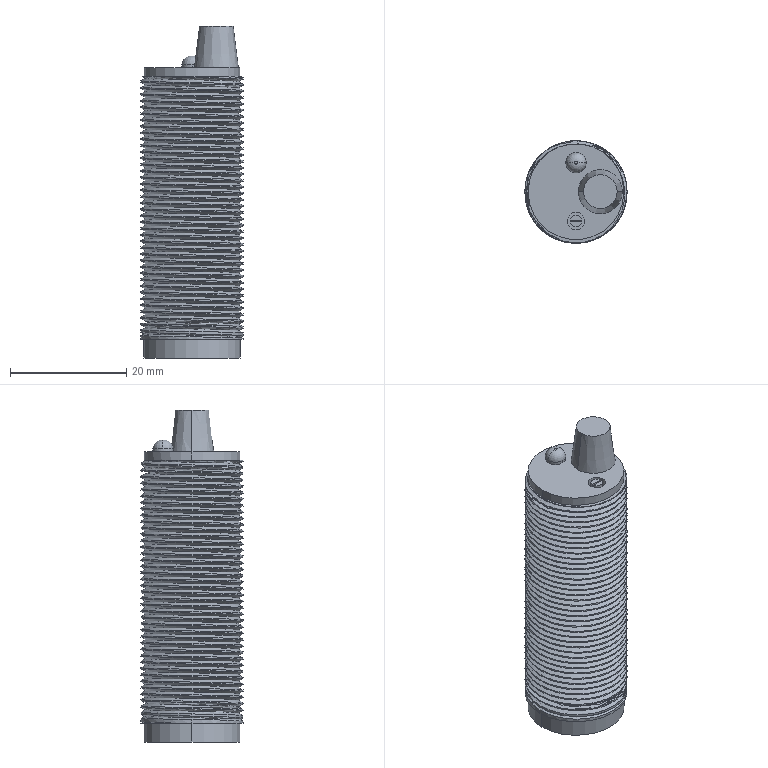Part | SolidWorks | features MBimport 1 | 1 solid | 126 faces | box 17.6 x 17.6 x 57.2 mm | volume 11322 mm3 | cylinder 100 | plane 16 | spline 6 | torus 2 | cone 2 | commonest cylinder face diameters 17.6 x84 16 x4 2 x2 3 x2 3.5 x2 14 x2